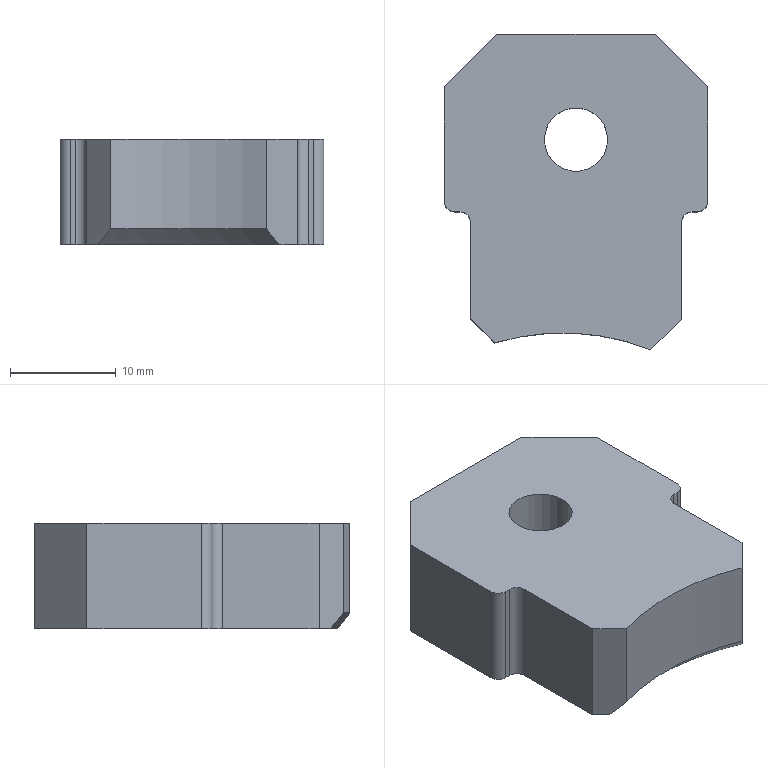Part | STEP file | solid 65 | 1 solid | 21 faces | box 25 x 29.916 x 10 mm | volume 5820 mm3 | plane 13 | cylinder 6 | cone 2 | commonest cylinder face diameters 2 x4 6 x1 45 x1